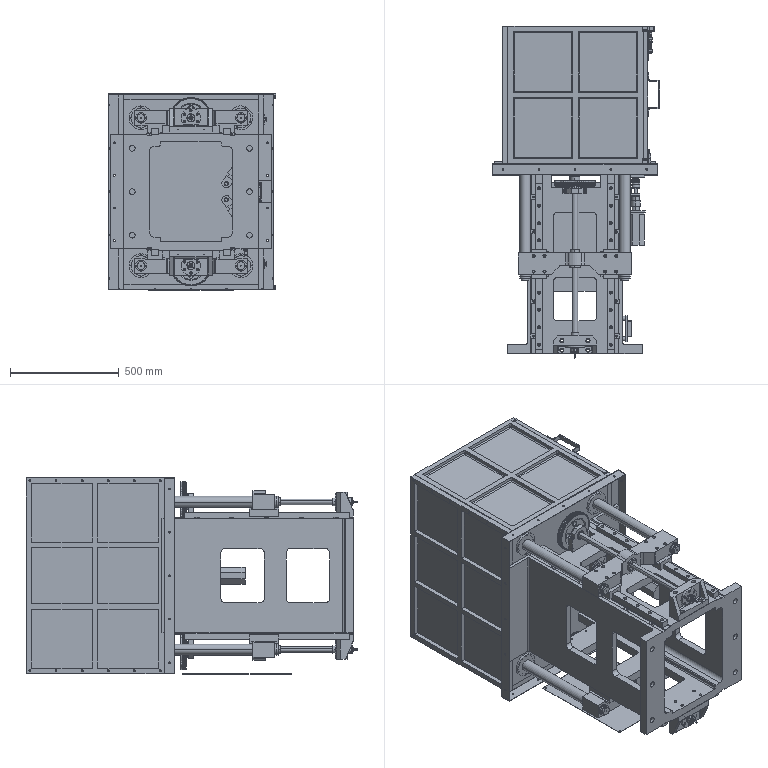Part | SolidWorks | features ReferencePattern 16, CompositeCurve 9, LocalLPattern 2 | 170 solids | 6022 faces | volume 100167004 mm3 | cylinder 3154 | plane 2125 | cone 579 | torus 138 | sphere 26 | commonest cylinder face diameters 0.8 x646 9 x218 4.2 x216 6 x173 10 x148 5 x124